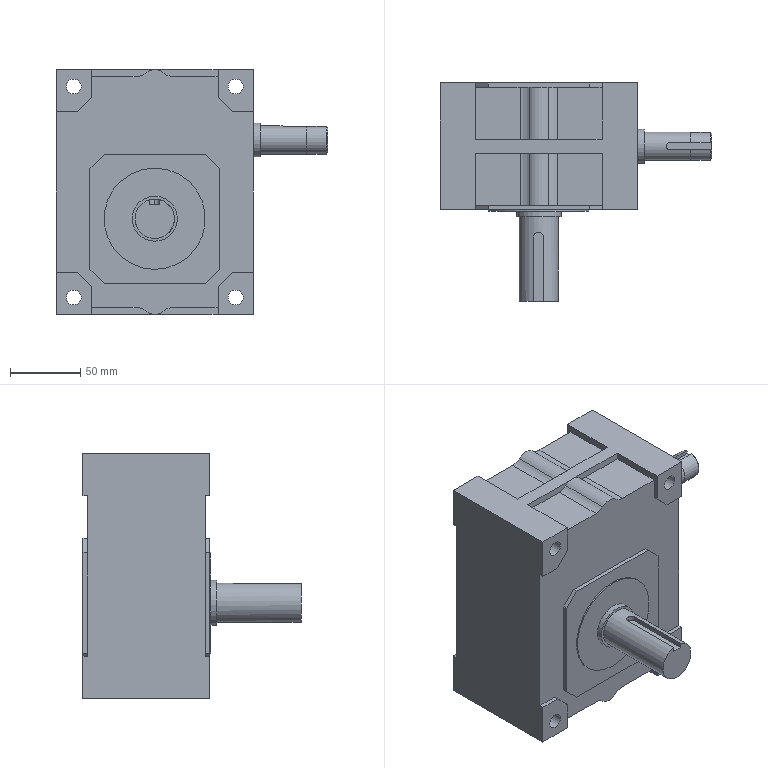Part | STEP file | YBQDJ-YB-20 | 1 solid | 109 faces | box 193 x 155 x 174 mm | volume 2083887 mm3 | plane 83 | cylinder 25 | cone 1 | commonest cylinder face diameters 20 x10 10.6 x4 20.262 x4 7 x2 5 x1 24 x1